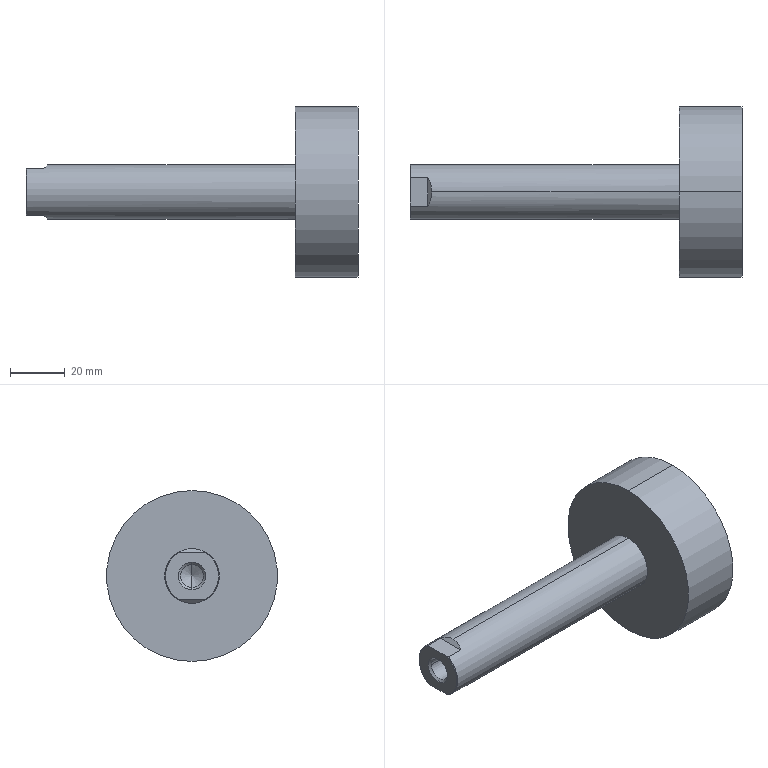Part | SolidWorks | features BaseBody 1 | 1 solid | 19 faces | box 121.5 x 62.5 x 62.5 mm | volume 100309 mm3 | plane 7 | cylinder 6 | cone 6 | commonest cylinder face diameters 8.376 x2 20 x2 62.5 x2
STEP:
#1=CARTESIAN_POINT('',(90.5,0.,10.));
#2=VERTEX_POINT('',#1);
#3=CARTESIAN_POINT('',(90.5,0.,-10.));
#4=VERTEX_POINT('',#3);
#5=CARTESIAN_POINT('',(90.5,0.,0.));
#6=DIRECTION('',(-1.,0.,0.));
#7=DIRECTION('',(0.,0.,1.));
#8=AXIS2_PLACEMENT_3D('',#5,#6,#7);
#9=CIRCLE('',#8,10.);
#10=EDGE_CURVE('',#2,#4,#9,.T.);
#11=ORIENTED_EDGE('',*,*,#10,.T.);
#12=CARTESIAN_POINT('',(0.,0.,-10.));
#13=VERTEX_POINT('',#12);
#14=CARTESIAN_POINT('',(0.,0.,-10.));
#15=DIRECTION('',(-1.,0.,0.));
#16=VECTOR('',#15,1000.);
#17=LINE('',#14,#16);
#18=EDGE_CURVE('',#4,#13,#17,.T.);
#19=ORIENTED_EDGE('',*,*,#18,.T.);
#20=CARTESIAN_POINT('',(-1.5,5.268,-8.5));
#21=VERTEX_POINT('',#20);
#22=CARTESIAN_POINT('',(0.,0.,-10.));
#23=CARTESIAN_POINT('',(0.,1.873,-10.));
#24=CARTESIAN_POINT('',(-0.5131,3.675,-9.487));
#25=CARTESIAN_POINT('',(-1.5,5.268,-8.5));
#26=(BOUNDED_CURVE()B_SPLINE_CURVE(3,(#22,#23,#24,#25),.UNSPECIFIED.,.F.,.F.)B_SPLINE_CURVE_WITH_KNOTS((4,4),(3.142,3.696),.UNSPECIFIED.)CURVE()GEOMETRIC_REPRESENTATION_ITEM()RATIONAL_B_SPLINE_CURVE((1.,0.9745,0.9745,1.))REPRESENTATION_ITEM(''));
#27=EDGE_CURVE('',#13,#21,#26,.T.);
#28=ORIENTED_EDGE('',*,*,#27,.T.);
#29=CARTESIAN_POINT('',(-7.75,5.268,-8.5));
#30=VERTEX_POINT('',#29);
#31=CARTESIAN_POINT('',(0.,5.268,-8.5));
#32=DIRECTION('',(-1.,0.,0.));
#33=VECTOR('',#32,1000.);
#34=LINE('',#31,#33);
#35=EDGE_CURVE('',#21,#30,#34,.T.);
#36=ORIENTED_EDGE('',*,*,#35,.T.);
#37=CARTESIAN_POINT('',(-7.75,5.268,8.5));
#38=VERTEX_POINT('',#37);
#39=CARTESIAN_POINT('',(-7.75,0.,0.));
#40=DIRECTION('',(1.,0.,0.));
#41=DIRECTION('',(0.,0.,1.));
#42=AXIS2_PLACEMENT_3D('',#39,#40,#41);
#43=CIRCLE('',#42,10.);
#44=EDGE_CURVE('',#30,#38,#43,.T.);
#45=ORIENTED_EDGE('',*,*,#44,.T.);
#46=CARTESIAN_POINT('',(-1.5,5.268,8.5));
#47=VERTEX_POINT('',#46);
#48=CARTESIAN_POINT('',(0.,5.268,8.5));
#49=DIRECTION('',(1.,0.,0.));
#50=VECTOR('',#49,1000.);
#51=LINE('',#48,#50);
#52=EDGE_CURVE('',#38,#47,#51,.T.);
#53=ORIENTED_EDGE('',*,*,#52,.T.);
#54=CARTESIAN_POINT('',(0.,0.,10.));
#55=VERTEX_POINT('',#54);
#56=CARTESIAN_POINT('',(-1.5,5.268,8.5));
#57=CARTESIAN_POINT('',(-0.5131,3.675,9.487));
#58=CARTESIAN_POINT('',(0.,1.873,10.));
#59=CARTESIAN_POINT('',(0.,0.,10.));
#60=(BOUNDED_CURVE()B_SPLINE_CURVE(3,(#56,#57,#58,#59),.UNSPECIFIED.,.F.,.F.)B_SPLINE_CURVE_WITH_KNOTS((4,4),(2.587,3.142),.UNSPECIFIED.)CURVE()GEOMETRIC_REPRESENTATION_ITEM()RATIONAL_B_SPLINE_CURVE((1.,0.9745,0.9745,1.))REPRESENTATION_ITEM(''));
#61=EDGE_CURVE('',#47,#55,#60,.T.);
#62=ORIENTED_EDGE('',*,*,#61,.T.);
#63=CARTESIAN_POINT('',(0.,0.,10.));
#64=DIRECTION('',(-1.,0.,0.));
#65=VECTOR('',#64,1000.);
#66=LINE('',#63,#65);
#67=EDGE_CURVE('',#2,#55,#66,.T.);
#68=ORIENTED_EDGE('',*,*,#67,.F.);
#69=EDGE_LOOP('',(#11,#19,#28,#36,#45,#53,#62,#68));
#70=FACE_OUTER_BOUND('',#69,.T.);
#71=CARTESIAN_POINT('',(0.,0.,0.));
#72=DIRECTION('',(-1.,0.,0.));
#73=DIRECTION('',(0.,0.,1.));
#74=AXIS2_PLACEMENT_3D('',#71,#72,#73);
#75=CYLINDRICAL_SURFACE('',#74,10.);
#76=ADVANCED_FACE('',(#70),#75,.T.);
#77=CARTESIAN_POINT('',(113.5,0.,31.25));
#78=VERTEX_POINT('',#77);
#79=CARTESIAN_POINT('',(113.5,0.,-31.25));
#80=VERTEX_POINT('',#79);
#81=CARTESIAN_POINT('',(113.5,0.,0.));
#82=DIRECTION('',(-1.,0.,0.));
#83=DIRECTION('',(0.,0.,1.));
#84=AXIS2_PLACEMENT_3D('',#81,#82,#83);
#85=CIRCLE('',#84,31.25);
#86=EDGE_CURVE('',#78,#80,#85,.T.);
#87=ORIENTED_EDGE('',*,*,#86,.T.);
#88=CARTESIAN_POINT('',(90.5,0.,-31.25));
#89=VERTEX_POINT('',#88);
#90=CARTESIAN_POINT('',(113.5,0.,-31.25));
#91=DIRECTION('',(-1.,0.,0.));
#92=VECTOR('',#91,1000.);
#93=LINE('',#90,#92);
#94=EDGE_CURVE('',#80,#89,#93,.T.);
#95=ORIENTED_EDGE('',*,*,#94,.T.);
#96=CARTESIAN_POINT('',(90.5,0.,31.25));
#97=VERTEX_POINT('',#96);
#98=CARTESIAN_POINT('',(90.5,0.,0.));
#99=DIRECTION('',(1.,0.,0.));
#100=DIRECTION('',(0.,0.,1.));
#101=AXIS2_PLACEMENT_3D('',#98,#99,#100);
#102=CIRCLE('',#101,31.25);
#103=EDGE_CURVE('',#89,#97,#102,.T.);
#104=ORIENTED_EDGE('',*,*,#103,.T.);
#105=CARTESIAN_POINT('',(113.5,0.,31.25));
#106=DIRECTION('',(-1.,0.,0.));
#107=VECTOR('',#106,1000.);
#108=LINE('',#105,#107);
#109=EDGE_CURVE('',#78,#97,#108,.T.);
#110=ORIENTED_EDGE('',*,*,#109,.F.);
#111=EDGE_LOOP('',(#87,#95,#104,#110));
#112=FACE_OUTER_BOUND('',#111,.T.);
#113=CARTESIAN_POINT('',(113.5,0.,0.));
#114=DIRECTION('',(-1.,0.,0.));
#115=DIRECTION('',(0.,0.,1.));
#116=AXIS2_PLACEMENT_3D('',#113,#114,#115);
#117=CYLINDRICAL_SURFACE('',#116,31.25);
#118=ADVANCED_FACE('',(#112),#117,.T.);
#119=CARTESIAN_POINT('',(-7.188,0.,-4.188));
#120=VERTEX_POINT('',#119);
#121=CARTESIAN_POINT('',(-7.188,-4.188,0.));
#122=VERTEX_POINT('',#121);
#123=CARTESIAN_POINT('',(-7.188,0.,0.));
#124=DIRECTION('',(-1.,0.,0.));
#125=DIRECTION('',(0.,-1.,0.));
#126=AXIS2_PLACEMENT_3D('',#123,#124,#125);
#127=CIRCLE('',#126,4.188);
#128=EDGE_CURVE('',#120,#122,#127,.T.);
#129=ORIENTED_EDGE('',*,*,#128,.F.);
#130=CARTESIAN_POINT('',(-8.,0.,-5.));
#131=VERTEX_POINT('',#130);
#132=CARTESIAN_POINT('',(-8.,0.,-5.));
#133=DIRECTION('',(-0.7071,0.,-0.7071));
#134=VECTOR('',#133,1000.);
#135=LINE('',#132,#134);
#136=EDGE_CURVE('',#120,#131,#135,.T.);
#137=ORIENTED_EDGE('',*,*,#136,.T.);
#138=CARTESIAN_POINT('',(-8.,0.,5.));
#139=VERTEX_POINT('',#138);
#140=CARTESIAN_POINT('',(-8.,0.,0.));
#141=DIRECTION('',(-1.,0.,0.));
#142=DIRECTION('',(0.,0.,1.));
#143=AXIS2_PLACEMENT_3D('',#140,#141,#142);
#144=CIRCLE('',#143,5.);
#145=EDGE_CURVE('',#131,#139,#144,.T.);
#146=ORIENTED_EDGE('',*,*,#145,.T.);
#147=CARTESIAN_POINT('',(-7.188,0.,4.188));
#148=VERTEX_POINT('',#147);
#149=CARTESIAN_POINT('',(-8.,0.,5.));
#150=DIRECTION('',(-0.7071,0.,0.7071));
#151=VECTOR('',#150,1000.);
#152=LINE('',#149,#151);
#153=EDGE_CURVE('',#148,#139,#152,.T.);
#154=ORIENTED_EDGE('',*,*,#153,.F.);
#155=CARTESIAN_POINT('',(-7.188,0.,0.));
#156=DIRECTION('',(-1.,0.,0.));
#157=DIRECTION('',(0.,-1.,0.));
#158=AXIS2_PLACEMENT_3D('',#155,#156,#157);
#159=CIRCLE('',#158,4.188);
#160=EDGE_CURVE('',#122,#148,#159,.T.);
#161=ORIENTED_EDGE('',*,*,#160,.F.);
#162=EDGE_LOOP('',(#129,#137,#146,#154,#161));
#163=FACE_OUTER_BOUND('',#162,.T.);
#164=CARTESIAN_POINT('',(-8.,0.,0.));
#165=DIRECTION('',(-1.,0.,0.));
#166=DIRECTION('',(0.,0.,1.));
#167=AXIS2_PLACEMENT_3D('',#164,#165,#166);
#168=CONICAL_SURFACE('',#167,5.,0.7854);
#169=ADVANCED_FACE('',(#163),#168,.F.);
#170=CARTESIAN_POINT('',(10.,4.188,0.));
#171=VERTEX_POINT('',#170);
#172=CARTESIAN_POINT('',(10.,0.,-4.188));
#173=VERTEX_POINT('',#172);
#174=CARTESIAN_POINT('',(10.,0.,0.));
#175=DIRECTION('',(-1.,0.,0.));
#176=DIRECTION('',(0.,-1.,0.));
#177=AXIS2_PLACEMENT_3D('',#174,#175,#176);
#178=CIRCLE('',#177,4.188);
#179=EDGE_CURVE('',#171,#173,#178,.T.);
#180=ORIENTED_EDGE('',*,*,#179,.F.);
#181=CARTESIAN_POINT('',(-7.188,4.188,0.));
#182=VERTEX_POINT('',#181);
#183=CARTESIAN_POINT('',(12.418,4.188,0.));
#184=DIRECTION('',(-1.,0.,0.));
#185=VECTOR('',#184,1000.);
#186=LINE('',#183,#185);
#187=EDGE_CURVE('',#171,#182,#186,.T.);
#188=ORIENTED_EDGE('',*,*,#187,.T.);
#189=CARTESIAN_POINT('',(-7.188,0.,0.));
#190=DIRECTION('',(-1.,0.,0.));
#191=DIRECTION('',(0.,-1.,0.));
#192=AXIS2_PLACEMENT_3D('',#189,#190,#191);
#193=CIRCLE('',#192,4.188);
#194=EDGE_CURVE('',#182,#120,#193,.T.);
#195=ORIENTED_EDGE('',*,*,#194,.T.);
#196=ORIENTED_EDGE('',*,*,#128,.T.);
#197=CARTESIAN_POINT('',(10.,-4.188,0.));
#198=VERTEX_POINT('',#197);
#199=CARTESIAN_POINT('',(12.418,-4.188,0.));
#200=DIRECTION('',(-1.,0.,0.));
#201=VECTOR('',#200,1000.);
#202=LINE('',#199,#201);
#203=EDGE_CURVE('',#198,#122,#202,.T.);
#204=ORIENTED_EDGE('',*,*,#203,.F.);
#205=CARTESIAN_POINT('',(10.,0.,0.));
#206=DIRECTION('',(-1.,0.,0.));
#207=DIRECTION('',(0.,-1.,0.));
#208=AXIS2_PLACEMENT_3D('',#205,#206,#207);
#209=CIRCLE('',#208,4.188);
#210=EDGE_CURVE('',#173,#198,#209,.T.);
#211=ORIENTED_EDGE('',*,*,#210,.F.);
#212=EDGE_LOOP('',(#180,#188,#195,#196,#204,#211));
#213=FACE_OUTER_BOUND('',#212,.T.);
#214=CARTESIAN_POINT('',(12.418,0.,0.));
#215=DIRECTION('',(-1.,0.,0.));
#216=DIRECTION('',(0.,-1.,0.));
#217=AXIS2_PLACEMENT_3D('',#214,#215,#216);
#218=CYLINDRICAL_SURFACE('',#217,4.188);
#219=ADVANCED_FACE('',(#213),#218,.F.);
#220=CARTESIAN_POINT('',(12.418,0.,0.));
#221=VERTEX_POINT('',#220);
#222=CARTESIAN_POINT('',(10.,0.,4.188));
#223=VERTEX_POINT('',#222);
#224=CARTESIAN_POINT('',(10.,0.,4.188));
#225=DIRECTION('',(-0.5,0.,0.866));
#226=VECTOR('',#225,1000.);
#227=LINE('',#224,#226);
#228=EDGE_CURVE('',#221,#223,#227,.T.);
#229=ORIENTED_EDGE('',*,*,#228,.F.);
#230=CARTESIAN_POINT('',(10.,0.,-4.188));
#231=DIRECTION('',(-0.5,0.,-0.866));
#232=VECTOR('',#231,1000.);
#233=LINE('',#230,#232);
#234=EDGE_CURVE('',#221,#173,#233,.T.);
#235=ORIENTED_EDGE('',*,*,#234,.T.);
#236=ORIENTED_EDGE('',*,*,#210,.T.);
#237=CARTESIAN_POINT('',(10.,0.,0.));
#238=DIRECTION('',(-1.,0.,0.));
#239=DIRECTION('',(0.,-1.,0.));
#240=AXIS2_PLACEMENT_3D('',#237,#238,#239);
#241=CIRCLE('',#240,4.188);
#242=EDGE_CURVE('',#198,#223,#241,.T.);
#243=ORIENTED_EDGE('',*,*,#242,.T.);
#244=EDGE_LOOP('',(#229,#235,#236,#243));
#245=FACE_OUTER_BOUND('',#244,.T.);
#246=CARTESIAN_POINT('',(10.,0.,0.));
#247=DIRECTION('',(-1.,0.,0.));
#248=DIRECTION('',(0.,0.,1.));
#249=AXIS2_PLACEMENT_3D('',#246,#247,#248);
#250=CONICAL_SURFACE('',#249,4.188,1.047);
#251=ADVANCED_FACE('',(#245),#250,.F.);
#252=ORIENTED_EDGE('',*,*,#18,.F.);
#253=CARTESIAN_POINT('',(90.5,0.,0.));
#254=DIRECTION('',(-1.,0.,0.));
#255=DIRECTION('',(0.,0.,1.));
#256=AXIS2_PLACEMENT_3D('',#253,#254,#255);
#257=CIRCLE('',#256,10.);
#258=EDGE_CURVE('',#4,#2,#257,.T.);
#259=ORIENTED_EDGE('',*,*,#258,.T.);
#260=ORIENTED_EDGE('',*,*,#67,.T.);
#261=CARTESIAN_POINT('',(-1.5,-5.268,8.5));
#262=VERTEX_POINT('',#261);
#263=CARTESIAN_POINT('',(0.,0.,10.));
#264=CARTESIAN_POINT('',(0.,-1.873,10.));
#265=CARTESIAN_POINT('',(-0.5131,-3.675,9.487));
#266=CARTESIAN_POINT('',(-1.5,-5.268,8.5));
#267=(BOUNDED_CURVE()B_SPLINE_CURVE(3,(#263,#264,#265,#266),.UNSPECIFIED.,.F.,.F.)B_SPLINE_CURVE_WITH_KNOTS((4,4),(3.142,3.696),.UNSPECIFIED.)CURVE()GEOMETRIC_REPRESENTATION_ITEM()RATIONAL_B_SPLINE_CURVE((1.,0.9745,0.9745,1.))REPRESENTATION_ITEM(''));
#268=EDGE_CURVE('',#55,#262,#267,.T.);
#269=ORIENTED_EDGE('',*,*,#268,.T.);
#270=CARTESIAN_POINT('',(-7.75,-5.268,8.5));
#271=VERTEX_POINT('',#270);
#272=CARTESIAN_POINT('',(0.,-5.268,8.5));
#273=DIRECTION('',(-1.,0.,0.));
#274=VECTOR('',#273,1000.);
#275=LINE('',#272,#274);
#276=EDGE_CURVE('',#262,#271,#275,.T.);
#277=ORIENTED_EDGE('',*,*,#276,.T.);
#278=CARTESIAN_POINT('',(-7.75,-5.268,-8.5));
#279=VERTEX_POINT('',#278);
#280=CARTESIAN_POINT('',(-7.75,0.,0.));
#281=DIRECTION('',(1.,0.,0.));
#282=DIRECTION('',(0.,0.,1.));
#283=AXIS2_PLACEMENT_3D('',#280,#281,#282);
#284=CIRCLE('',#283,10.);
#285=EDGE_CURVE('',#271,#279,#284,.T.);
#286=ORIENTED_EDGE('',*,*,#285,.T.);
#287=CARTESIAN_POINT('',(-1.5,-5.268,-8.5));
#288=VERTEX_POINT('',#287);
#289=CARTESIAN_POINT('',(0.,-5.268,-8.5));
#290=DIRECTION('',(1.,0.,0.));
#291=VECTOR('',#290,1000.);
#292=LINE('',#289,#291);
#293=EDGE_CURVE('',#279,#288,#292,.T.);
#294=ORIENTED_EDGE('',*,*,#293,.T.);
#295=CARTESIAN_POINT('',(-1.5,-5.268,-8.5));
#296=CARTESIAN_POINT('',(-0.5131,-3.675,-9.487));
#297=CARTESIAN_POINT('',(0.,-1.873,-10.));
#298=CARTESIAN_POINT('',(0.,0.,-10.));
#299=(BOUNDED_CURVE()B_SPLINE_CURVE(3,(#295,#296,#297,#298),.UNSPECIFIED.,.F.,.F.)B_SPLINE_CURVE_WITH_KNOTS((4,4),(2.587,3.142),.UNSPECIFIED.)CURVE()GEOMETRIC_REPRESENTATION_ITEM()RATIONAL_B_SPLINE_CURVE((1.,0.9745,0.9745,1.))REPRESENTATION_ITEM(''));
#300=EDGE_CURVE('',#288,#13,#299,.T.);
#301=ORIENTED_EDGE('',*,*,#300,.T.);
#302=EDGE_LOOP('',(#252,#259,#260,#269,#277,#286,#294,#301));
#303=FACE_OUTER_BOUND('',#302,.T.);
#304=CARTESIAN_POINT('',(0.,0.,0.));
#305=DIRECTION('',(-1.,0.,0.));
#306=DIRECTION('',(0.,0.,1.));
#307=AXIS2_PLACEMENT_3D('',#304,#305,#306);
#308=CYLINDRICAL_SURFACE('',#307,10.);
#309=ADVANCED_FACE('',(#303),#308,.T.);
#310=ORIENTED_EDGE('',*,*,#61,.F.);
#311=CARTESIAN_POINT('',(-1.5,17.,8.5));
#312=DIRECTION('',(0.,-1.,0.));
#313=VECTOR('',#312,1000.);
#314=LINE('',#311,#313);
#315=EDGE_CURVE('',#47,#262,#314,.T.);
#316=ORIENTED_EDGE('',*,*,#315,.T.);
#317=ORIENTED_EDGE('',*,*,#268,.F.);
#318=EDGE_LOOP('',(#310,#316,#317));
#319=FACE_OUTER_BOUND('',#318,.T.);
#320=CARTESIAN_POINT('',(3.5,17.,13.5));
#321=DIRECTION('',(-0.7071,0.,0.7071));
#322=DIRECTION('',(0.7071,0.,0.7071));
#323=AXIS2_PLACEMENT_3D('',#320,#321,#322);
#324=PLANE('',#323);
#325=ADVANCED_FACE('',(#319),#324,.T.);
#326=CARTESIAN_POINT('',(-8.,4.776,8.5));
#327=VERTEX_POINT('',#326);
#328=CARTESIAN_POINT('',(-7.75,5.268,8.5));
#329=CARTESIAN_POINT('',(-7.837,5.102,8.5));
#330=CARTESIAN_POINT('',(-7.921,4.938,8.5));
#331=CARTESIAN_POINT('',(-8.,4.776,8.5));
#332=B_SPLINE_CURVE_WITH_KNOTS('',3,(#328,#329,#330,#331),.UNSPECIFIED.,.F.,.F.,(4,4),(0.,1.),.UNSPECIFIED.);
#333=EDGE_CURVE('',#38,#327,#332,.T.);
#334=ORIENTED_EDGE('',*,*,#333,.T.);
#335=CARTESIAN_POINT('',(-8.,-4.776,8.5));
#336=VERTEX_POINT('',#335);
#337=CARTESIAN_POINT('',(-8.,17.,8.5));
#338=DIRECTION('',(0.,-1.,0.));
#339=VECTOR('',#338,1000.);
#340=LINE('',#337,#339);
#341=EDGE_CURVE('',#327,#336,#340,.T.);
#342=ORIENTED_EDGE('',*,*,#341,.T.);
#343=CARTESIAN_POINT('',(-8.,-4.776,8.5));
#344=CARTESIAN_POINT('',(-7.921,-4.938,8.5));
#345=CARTESIAN_POINT('',(-7.837,-5.102,8.5));
#346=CARTESIAN_POINT('',(-7.75,-5.268,8.5));
#347=B_SPLINE_CURVE_WITH_KNOTS('',3,(#343,#344,#345,#346),.UNSPECIFIED.,.F.,.F.,(4,4),(0.,1.),.UNSPECIFIED.);
#348=EDGE_CURVE('',#336,#271,#347,.T.);
#349=ORIENTED_EDGE('',*,*,#348,.T.);
#350=ORIENTED_EDGE('',*,*,#276,.F.);
#351=ORIENTED_EDGE('',*,*,#315,.F.);
#352=ORIENTED_EDGE('',*,*,#52,.F.);
#353=EDGE_LOOP('',(#334,#342,#349,#350,#351,#352));
#354=FACE_OUTER_BOUND('',#353,.T.);
#355=CARTESIAN_POINT('',(-1.5,17.,8.5));
#356=DIRECTION('',(0.,0.,1.));
#357=DIRECTION('',(1.,0.,0.));
#358=AXIS2_PLACEMENT_3D('',#355,#356,#357);
#359=PLANE('',#358);
#360=ADVANCED_FACE('',(#354),#359,.T.);
#361=ORIENTED_EDGE('',*,*,#333,.F.);
#362=ORIENTED_EDGE('',*,*,#44,.F.);
#363=CARTESIAN_POINT('',(-8.,4.776,-8.5));
#364=VERTEX_POINT('',#363);
#365=CARTESIAN_POINT('',(-7.75,5.268,-8.5));
#366=CARTESIAN_POINT('',(-7.837,5.103,-8.5));
#367=CARTESIAN_POINT('',(-7.92,4.939,-8.5));
#368=CARTESIAN_POINT('',(-8.,4.776,-8.5));
#369=B_SPLINE_CURVE_WITH_KNOTS('',3,(#365,#366,#367,#368),.UNSPECIFIED.,.F.,.F.,(4,4),(0.,1.),.UNSPECIFIED.);
#370=EDGE_CURVE('',#30,#364,#369,.T.);
#371=ORIENTED_EDGE('',*,*,#370,.T.);
#372=CARTESIAN_POINT('',(-8.,0.,0.));
#373=DIRECTION('',(1.,0.,0.));
#374=DIRECTION('',(0.,0.,-1.));
#375=AXIS2_PLACEMENT_3D('',#372,#373,#374);
#376=CIRCLE('',#375,9.75);
#377=EDGE_CURVE('',#364,#327,#376,.T.);
#378=ORIENTED_EDGE('',*,*,#377,.T.);
#379=EDGE_LOOP('',(#361,#362,#371,#378));
#380=FACE_OUTER_BOUND('',#379,.T.);
#381=CARTESIAN_POINT('',(-7.75,0.,0.));
#382=DIRECTION('',(1.,0.,0.));
#383=DIRECTION('',(0.,0.,-1.));
#384=AXIS2_PLACEMENT_3D('',#381,#382,#383);
#385=CONICAL_SURFACE('',#384,10.,0.7854);
#386=ADVANCED_FACE('',(#380),#385,.T.);
#387=CARTESIAN_POINT('',(-8.,-4.776,-8.5));
#388=VERTEX_POINT('',#387);
#389=CARTESIAN_POINT('',(-7.75,-5.268,-8.5));
#390=CARTESIAN_POINT('',(-7.837,-5.102,-8.5));
#391=CARTESIAN_POINT('',(-7.921,-4.938,-8.5));
#392=CARTESIAN_POINT('',(-8.,-4.776,-8.5));
#393=B_SPLINE_CURVE_WITH_KNOTS('',3,(#389,#390,#391,#392),.UNSPECIFIED.,.F.,.F.,(4,4),(0.,1.),.UNSPECIFIED.);
#394=EDGE_CURVE('',#279,#388,#393,.T.);
#395=ORIENTED_EDGE('',*,*,#394,.T.);
#396=CARTESIAN_POINT('',(-8.,17.,-8.5));
#397=DIRECTION('',(0.,1.,0.));
#398=VECTOR('',#397,1000.);
#399=LINE('',#396,#398);
#400=EDGE_CURVE('',#388,#364,#399,.T.);
#401=ORIENTED_EDGE('',*,*,#400,.T.);
#402=ORIENTED_EDGE('',*,*,#370,.F.);
#403=ORIENTED_EDGE('',*,*,#35,.F.);
#404=CARTESIAN_POINT('',(-1.5,17.,-8.5));
#405=DIRECTION('',(0.,-1.,0.));
#406=VECTOR('',#405,1000.);
#407=LINE('',#404,#406);
#408=EDGE_CURVE('',#21,#288,#407,.T.);
#409=ORIENTED_EDGE('',*,*,#408,.T.);
#410=ORIENTED_EDGE('',*,*,#293,.F.);
#411=EDGE_LOOP('',(#395,#401,#402,#403,#409,#410));
#412=FACE_OUTER_BOUND('',#411,.T.);
#413=CARTESIAN_POINT('',(-8.,17.,-8.5));
#414=DIRECTION('',(0.,0.,-1.));
#415=DIRECTION('',(-1.,0.,0.));
#416=AXIS2_PLACEMENT_3D('',#413,#414,#415);
#417=PLANE('',#416);
#418=ADVANCED_FACE('',(#412),#417,.T.);
#419=ORIENTED_EDGE('',*,*,#300,.F.);
#420=ORIENTED_EDGE('',*,*,#408,.F.);
#421=ORIENTED_EDGE('',*,*,#27,.F.);
#422=EDGE_LOOP('',(#419,#420,#421));
#423=FACE_OUTER_BOUND('',#422,.T.);
#424=CARTESIAN_POINT('',(-1.5,17.,-8.5));
#425=DIRECTION('',(-0.7071,0.,-0.7071));
#426=DIRECTION('',(-0.7071,0.,0.7071));
#427=AXIS2_PLACEMENT_3D('',#424,#425,#426);
#428=PLANE('',#427);
#429=ADVANCED_FACE('',(#423),#428,.T.);
#430=ORIENTED_EDGE('',*,*,#394,.F.);
#431=ORIENTED_EDGE('',*,*,#285,.F.);
#432=ORIENTED_EDGE('',*,*,#348,.F.);
#433=CARTESIAN_POINT('',(-8.,0.,0.));
#434=DIRECTION('',(1.,0.,0.));
#435=DIRECTION('',(0.,0.,-1.));
#436=AXIS2_PLACEMENT_3D('',#433,#434,#435);
#437=CIRCLE('',#436,9.75);
#438=EDGE_CURVE('',#336,#388,#437,.T.);
#439=ORIENTED_EDGE('',*,*,#438,.T.);
#440=EDGE_LOOP('',(#430,#431,#432,#439));
#441=FACE_OUTER_BOUND('',#440,.T.);
#442=CARTESIAN_POINT('',(-7.75,0.,0.));
#443=DIRECTION('',(1.,0.,0.));
#444=DIRECTION('',(0.,0.,-1.));
#445=AXIS2_PLACEMENT_3D('',#442,#443,#444);
#446=CONICAL_SURFACE('',#445,10.,0.7854);
#447=ADVANCED_FACE('',(#441),#446,.T.);
#448=ORIENTED_EDGE('',*,*,#10,.F.);
#449=ORIENTED_EDGE('',*,*,#258,.F.);
#450=EDGE_LOOP('',(#448,#449));
#451=FACE_BOUND('',#450,.T.);
#452=CARTESIAN_POINT('',(90.5,0.,0.));
#453=DIRECTION('',(1.,0.,0.));
#454=DIRECTION('',(0.,0.,1.));
#455=AXIS2_PLACEMENT_3D('',#452,#453,#454);
#456=CIRCLE('',#455,31.25);
#457=EDGE_CURVE('',#97,#89,#456,.T.);
#458=ORIENTED_EDGE('',*,*,#457,.F.);
#459=ORIENTED_EDGE('',*,*,#103,.F.);
#460=EDGE_LOOP('',(#458,#459));
#461=FACE_OUTER_BOUND('',#460,.T.);
#462=CARTESIAN_POINT('',(90.5,10.,0.));
#463=DIRECTION('',(1.,0.,0.));
#464=DIRECTION('',(0.,0.,-1.));
#465=AXIS2_PLACEMENT_3D('',#462,#463,#464);
#466=PLANE('',#465);
#467=ADVANCED_FACE('',(#451,#461),#466,.F.);
#468=CARTESIAN_POINT('',(-8.,0.,0.));
#469=DIRECTION('',(-1.,0.,0.));
#470=DIRECTION('',(0.,0.,1.));
#471=AXIS2_PLACEMENT_3D('',#468,#469,#470);
#472=CIRCLE('',#471,5.);
#473=EDGE_CURVE('',#139,#131,#472,.T.);
#474=ORIENTED_EDGE('',*,*,#473,.F.);
#475=ORIENTED_EDGE('',*,*,#145,.F.);
#476=EDGE_LOOP('',(#474,#475));
#477=FACE_BOUND('',#476,.T.);
#478=ORIENTED_EDGE('',*,*,#400,.F.);
#479=ORIENTED_EDGE('',*,*,#438,.F.);
#480=ORIENTED_EDGE('',*,*,#341,.F.);
#481=ORIENTED_EDGE('',*,*,#377,.F.);
#482=EDGE_LOOP('',(#478,#479,#480,#481));
#483=FACE_OUTER_BOUND('',#482,.T.);
#484=CARTESIAN_POINT('',(-8.,0.,0.));
#485=DIRECTION('',(1.,0.,0.));
#486=DIRECTION('',(0.,0.,-1.));
#487=AXIS2_PLACEMENT_3D('',#484,#485,#486);
#488=PLANE('',#487);
#489=ADVANCED_FACE('',(#477,#483),#488,.F.);
#490=ORIENTED_EDGE('',*,*,#94,.F.);
#491=CARTESIAN_POINT('',(113.5,0.,0.));
#492=DIRECTION('',(-1.,0.,0.));
#493=DIRECTION('',(0.,0.,1.));
#494=AXIS2_PLACEMENT_3D('',#491,#492,#493);
#495=CIRCLE('',#494,31.25);
#496=EDGE_CURVE('',#80,#78,#495,.T.);
#497=ORIENTED_EDGE('',*,*,#496,.T.);
#498=ORIENTED_EDGE('',*,*,#109,.T.);
#499=ORIENTED_EDGE('',*,*,#457,.T.);
#500=EDGE_LOOP('',(#490,#497,#498,#499));
#501=FACE_OUTER_BOUND('',#500,.T.);
#502=CARTESIAN_POINT('',(113.5,0.,0.));
#503=DIRECTION('',(-1.,0.,0.));
#504=DIRECTION('',(0.,0.,1.));
#505=AXIS2_PLACEMENT_3D('',#502,#503,#504);
#506=CYLINDRICAL_SURFACE('',#505,31.25);
#507=ADVANCED_FACE('',(#501),#506,.T.);
#508=ORIENTED_EDGE('',*,*,#136,.F.);
#509=ORIENTED_EDGE('',*,*,#194,.F.);
#510=CARTESIAN_POINT('',(-7.188,0.,0.));
#511=DIRECTION('',(-1.,0.,0.));
#512=DIRECTION('',(0.,-1.,0.));
#513=AXIS2_PLACEMENT_3D('',#510,#511,#512);
#514=CIRCLE('',#513,4.188);
#515=EDGE_CURVE('',#148,#182,#514,.T.);
#516=ORIENTED_EDGE('',*,*,#515,.F.);
#517=ORIENTED_EDGE('',*,*,#153,.T.);
#518=ORIENTED_EDGE('',*,*,#473,.T.);
#519=EDGE_LOOP('',(#508,#509,#516,#517,#518));
#520=FACE_OUTER_BOUND('',#519,.T.);
#521=CARTESIAN_POINT('',(-8.,0.,0.));
#522=DIRECTION('',(-1.,0.,0.));
#523=DIRECTION('',(0.,0.,1.));
#524=AXIS2_PLACEMENT_3D('',#521,#522,#523);
#525=CONICAL_SURFACE('',#524,5.,0.7854);
#526=ADVANCED_FACE('',(#520),#525,.F.);
#527=ORIENTED_EDGE('',*,*,#86,.F.);
#528=ORIENTED_EDGE('',*,*,#496,.F.);
#529=EDGE_LOOP('',(#527,#528));
#530=FACE_OUTER_BOUND('',#529,.T.);
#531=CARTESIAN_POINT('',(113.5,31.25,0.));
#532=DIRECTION('',(-1.,0.,0.));
#533=DIRECTION('',(0.,0.,1.));
#534=AXIS2_PLACEMENT_3D('',#531,#532,#533);
#535=PLANE('',#534);
#536=ADVANCED_FACE('',(#530),#535,.F.);
#537=ORIENTED_EDGE('',*,*,#187,.F.);
#538=CARTESIAN_POINT('',(10.,0.,0.));
#539=DIRECTION('',(-1.,0.,0.));
#540=DIRECTION('',(0.,-1.,0.));
#541=AXIS2_PLACEMENT_3D('',#538,#539,#540);
#542=CIRCLE('',#541,4.188);
#543=EDGE_CURVE('',#223,#171,#542,.T.);
#544=ORIENTED_EDGE('',*,*,#543,.F.);
#545=ORIENTED_EDGE('',*,*,#242,.F.);
#546=ORIENTED_EDGE('',*,*,#203,.T.);
#547=ORIENTED_EDGE('',*,*,#160,.T.);
#548=ORIENTED_EDGE('',*,*,#515,.T.);
#549=EDGE_LOOP('',(#537,#544,#545,#546,#547,#548));
#550=FACE_OUTER_BOUND('',#549,.T.);
#551=CARTESIAN_POINT('',(12.418,0.,0.));
#552=DIRECTION('',(-1.,0.,0.));
#553=DIRECTION('',(0.,-1.,0.));
#554=AXIS2_PLACEMENT_3D('',#551,#552,#553);
#555=CYLINDRICAL_SURFACE('',#554,4.188);
#556=ADVANCED_FACE('',(#550),#555,.F.);
#557=ORIENTED_EDGE('',*,*,#234,.F.);
#558=ORIENTED_EDGE('',*,*,#228,.T.);
#559=ORIENTED_EDGE('',*,*,#543,.T.);
#560=ORIENTED_EDGE('',*,*,#179,.T.);
#561=EDGE_LOOP('',(#557,#558,#559,#560));
#562=FACE_OUTER_BOUND('',#561,.T.);
#563=CARTESIAN_POINT('',(10.,0.,0.));
#564=DIRECTION('',(-1.,0.,0.));
#565=DIRECTION('',(0.,0.,1.));
#566=AXIS2_PLACEMENT_3D('',#563,#564,#565);
#567=CONICAL_SURFACE('',#566,4.188,1.047);
#568=ADVANCED_FACE('',(#562),#567,.F.);
#569=CLOSED_SHELL('',(#76,#118,#169,#219,#251,#309,#325,#360,#386,#418,#429,#447,#467,#489,#507,#526,#536,#556,#568));
#570=MANIFOLD_SOLID_BREP('',#569);
#571=CARTESIAN_POINT('',(0.,0.,0.));
#572=DIRECTION('',(0.,0.,1.));
#573=DIRECTION('',(1.,0.,0.));
#574=AXIS2_PLACEMENT_3D('',#571,#572,#573);
#575=(LENGTH_UNIT()NAMED_UNIT(*)SI_UNIT(.MILLI.,.METRE.));
#576=UNCERTAINTY_MEASURE_WITH_UNIT(LENGTH_MEASURE(0.00001),#575,'','');
#577=(NAMED_UNIT(*)PLANE_ANGLE_UNIT()SI_UNIT($,.RADIAN.));
#578=(NAMED_UNIT(*)SI_UNIT($,.STERADIAN.)SOLID_ANGLE_UNIT());
#579=(GEOMETRIC_REPRESENTATION_CONTEXT(3)GLOBAL_UNCERTAINTY_ASSIGNED_CONTEXT((#576))GLOBAL_UNIT_ASSIGNED_CONTEXT((#575,#577,#578))REPRESENTATION_CONTEXT('',''));
#580=ADVANCED_BREP_SHAPE_REPRESENTATION('',(#570,#574),#579);